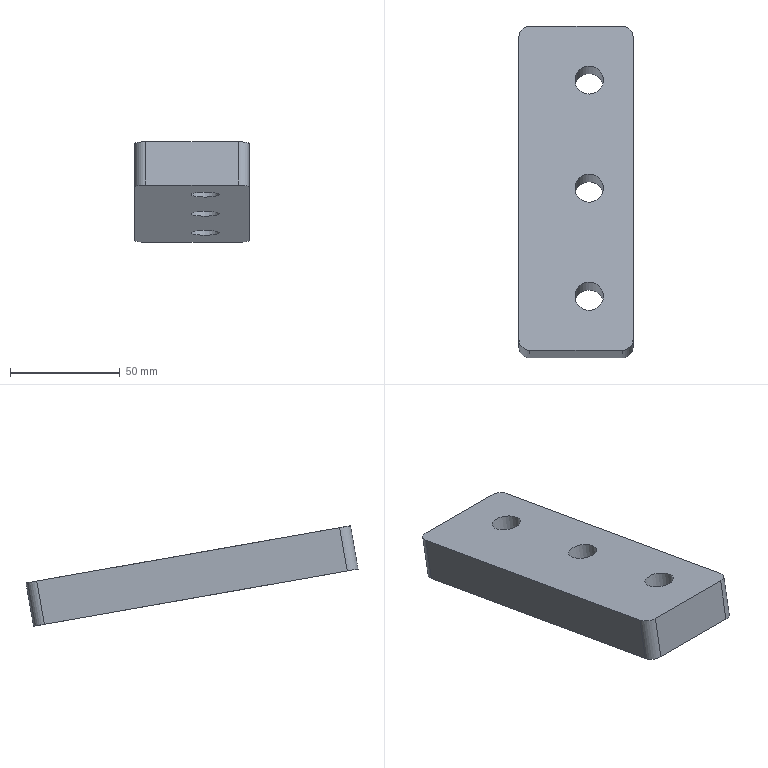Part | NX | features MAIN_BODY 2 | 1 solid | 13 faces | box 52 x 151.194 x 45.743 mm | volume 147607 mm3 | cylinder 7 | plane 6 | commonest cylinder face diameters 10 x4 13 x3
STEP:
#1=CARTESIAN_POINT('',(868.762,-740.098,-73.129));
#2=VERTEX_POINT('',#1);
#3=CARTESIAN_POINT('',(910.762,-740.098,-73.129));
#4=VERTEX_POINT('',#3);
#5=CARTESIAN_POINT('',(863.762,-740.098,-73.129));
#6=DIRECTION('',(1.,0.,0.));
#7=VECTOR('',#6,1000.);
#8=LINE('',#5,#7);
#9=EDGE_CURVE('',#2,#4,#8,.T.);
#10=ORIENTED_EDGE('',*,*,#9,.F.);
#11=CARTESIAN_POINT('',(868.762,-736.625,-53.433));
#12=VERTEX_POINT('',#11);
#13=CARTESIAN_POINT('',(868.762,-736.625,-53.433));
#14=DIRECTION('',(0.,-0.1736,-0.9848));
#15=VECTOR('',#14,1000.);
#16=LINE('',#13,#15);
#17=EDGE_CURVE('',#2,#12,#16,.F.);
#18=ORIENTED_EDGE('',*,*,#17,.T.);
#19=CARTESIAN_POINT('',(910.762,-736.625,-53.433));
#20=VERTEX_POINT('',#19);
#21=CARTESIAN_POINT('',(863.762,-736.625,-53.433));
#22=DIRECTION('',(1.,0.,0.));
#23=VECTOR('',#22,1000.);
#24=LINE('',#21,#23);
#25=EDGE_CURVE('',#12,#20,#24,.T.);
#26=ORIENTED_EDGE('',*,*,#25,.T.);
#27=CARTESIAN_POINT('',(910.762,-736.625,-53.433));
#28=DIRECTION('',(0.,-0.1736,-0.9848));
#29=VECTOR('',#28,1000.);
#30=LINE('',#27,#29);
#31=EDGE_CURVE('',#20,#4,#30,.T.);
#32=ORIENTED_EDGE('',*,*,#31,.T.);
#33=EDGE_LOOP('',(#10,#18,#26,#32));
#34=FACE_BOUND('',#33,.T.);
#35=CARTESIAN_POINT('',(863.762,-736.625,-53.433));
#36=DIRECTION('',(0.,0.9848,-0.1736));
#37=DIRECTION('',(-1.,0.,0.));
#38=AXIS2_PLACEMENT_3D('',#35,#36,#37);
#39=PLANE('',#38);
#40=ADVANCED_FACE('',(#34),#39,.T.);
#41=CARTESIAN_POINT('',(915.762,-745.022,-72.261));
#42=VERTEX_POINT('',#41);
#43=CARTESIAN_POINT('',(915.762,-882.895,-47.95));
#44=VERTEX_POINT('',#43);
#45=CARTESIAN_POINT('',(915.762,-740.098,-73.129));
#46=DIRECTION('',(0.,-0.9848,0.1736));
#47=VECTOR('',#46,1000.);
#48=LINE('',#45,#47);
#49=EDGE_CURVE('',#42,#44,#48,.T.);
#50=ORIENTED_EDGE('',*,*,#49,.F.);
#51=CARTESIAN_POINT('',(915.762,-741.549,-52.564));
#52=VERTEX_POINT('',#51);
#53=CARTESIAN_POINT('',(915.762,-741.549,-52.564));
#54=DIRECTION('',(0.,-0.1736,-0.9848));
#55=VECTOR('',#54,1000.);
#56=LINE('',#53,#55);
#57=EDGE_CURVE('',#42,#52,#56,.F.);
#58=ORIENTED_EDGE('',*,*,#57,.T.);
#59=CARTESIAN_POINT('',(915.762,-879.422,-28.254));
#60=VERTEX_POINT('',#59);
#61=CARTESIAN_POINT('',(915.762,-736.625,-53.433));
#62=DIRECTION('',(0.,-0.9848,0.1736));
#63=VECTOR('',#62,1000.);
#64=LINE('',#61,#63);
#65=EDGE_CURVE('',#52,#60,#64,.T.);
#66=ORIENTED_EDGE('',*,*,#65,.T.);
#67=CARTESIAN_POINT('',(915.762,-879.422,-28.254));
#68=DIRECTION('',(0.,-0.1736,-0.9848));
#69=VECTOR('',#68,1000.);
#70=LINE('',#67,#69);
#71=EDGE_CURVE('',#60,#44,#70,.T.);
#72=ORIENTED_EDGE('',*,*,#71,.T.);
#73=EDGE_LOOP('',(#50,#58,#66,#72));
#74=FACE_BOUND('',#73,.T.);
#75=CARTESIAN_POINT('',(915.762,-736.625,-53.433));
#76=DIRECTION('',(1.,0.,0.));
#77=DIRECTION('',(0.,0.9848,-0.1736));
#78=AXIS2_PLACEMENT_3D('',#75,#76,#77);
#79=PLANE('',#78);
#80=ADVANCED_FACE('',(#74),#79,.T.);
#81=CARTESIAN_POINT('',(863.762,-879.422,-28.254));
#82=VERTEX_POINT('',#81);
#83=CARTESIAN_POINT('',(863.762,-741.549,-52.564));
#84=VERTEX_POINT('',#83);
#85=CARTESIAN_POINT('',(863.762,-810.485,-40.409));
#86=DIRECTION('',(0.,0.9848,-0.1736));
#87=VECTOR('',#86,1000.);
#88=LINE('',#85,#87);
#89=EDGE_CURVE('',#82,#84,#88,.T.);
#90=ORIENTED_EDGE('',*,*,#89,.T.);
#91=CARTESIAN_POINT('',(863.762,-745.022,-72.261));
#92=VERTEX_POINT('',#91);
#93=CARTESIAN_POINT('',(863.762,-741.549,-52.564));
#94=DIRECTION('',(0.,-0.1736,-0.9848));
#95=VECTOR('',#94,1000.);
#96=LINE('',#93,#95);
#97=EDGE_CURVE('',#84,#92,#96,.T.);
#98=ORIENTED_EDGE('',*,*,#97,.T.);
#99=CARTESIAN_POINT('',(863.762,-882.895,-47.95));
#100=VERTEX_POINT('',#99);
#101=CARTESIAN_POINT('',(863.762,-813.958,-60.105));
#102=DIRECTION('',(0.,0.9848,-0.1736));
#103=VECTOR('',#102,1000.);
#104=LINE('',#101,#103);
#105=EDGE_CURVE('',#100,#92,#104,.T.);
#106=ORIENTED_EDGE('',*,*,#105,.F.);
#107=CARTESIAN_POINT('',(863.762,-879.422,-28.254));
#108=DIRECTION('',(0.,-0.1736,-0.9848));
#109=VECTOR('',#108,1000.);
#110=LINE('',#107,#109);
#111=EDGE_CURVE('',#100,#82,#110,.F.);
#112=ORIENTED_EDGE('',*,*,#111,.T.);
#113=EDGE_LOOP('',(#90,#98,#106,#112));
#114=FACE_BOUND('',#113,.T.);
#115=CARTESIAN_POINT('',(863.762,-810.485,-40.409));
#116=DIRECTION('',(-1.,0.,0.));
#117=DIRECTION('',(0.,-0.9848,0.1736));
#118=AXIS2_PLACEMENT_3D('',#115,#116,#117);
#119=PLANE('',#118);
#120=ADVANCED_FACE('',(#114),#119,.T.);
#121=ORIENTED_EDGE('',*,*,#25,.F.);
#122=CARTESIAN_POINT('',(868.762,-741.549,-52.564));
#123=DIRECTION('',(0.,-0.1736,-0.9848));
#124=DIRECTION('',(0.,-0.9848,0.1736));
#125=AXIS2_PLACEMENT_3D('',#122,#123,#124);
#126=CIRCLE('',#125,5.);
#127=EDGE_CURVE('',#12,#84,#126,.F.);
#128=ORIENTED_EDGE('',*,*,#127,.T.);
#129=ORIENTED_EDGE('',*,*,#89,.F.);
#130=CARTESIAN_POINT('',(868.762,-884.346,-27.385));
#131=VERTEX_POINT('',#130);
#132=CARTESIAN_POINT('',(868.762,-879.422,-28.254));
#133=DIRECTION('',(0.,-0.1736,-0.9848));
#134=DIRECTION('',(0.,-0.9848,0.1736));
#135=AXIS2_PLACEMENT_3D('',#132,#133,#134);
#136=CIRCLE('',#135,5.);
#137=EDGE_CURVE('',#82,#131,#136,.F.);
#138=ORIENTED_EDGE('',*,*,#137,.T.);
#139=CARTESIAN_POINT('',(910.762,-884.346,-27.385));
#140=VERTEX_POINT('',#139);
#141=CARTESIAN_POINT('',(863.762,-884.346,-27.385));
#142=DIRECTION('',(1.,0.,0.));
#143=VECTOR('',#142,1000.);
#144=LINE('',#141,#143);
#145=EDGE_CURVE('',#131,#140,#144,.T.);
#146=ORIENTED_EDGE('',*,*,#145,.T.);
#147=CARTESIAN_POINT('',(910.762,-879.422,-28.254));
#148=DIRECTION('',(0.,-0.1736,-0.9848));
#149=DIRECTION('',(0.,-0.9848,0.1736));
#150=AXIS2_PLACEMENT_3D('',#147,#148,#149);
#151=CIRCLE('',#150,5.);
#152=EDGE_CURVE('',#140,#60,#151,.F.);
#153=ORIENTED_EDGE('',*,*,#152,.T.);
#154=ORIENTED_EDGE('',*,*,#65,.F.);
#155=CARTESIAN_POINT('',(910.762,-741.549,-52.564));
#156=DIRECTION('',(0.,-0.1736,-0.9848));
#157=DIRECTION('',(0.,-0.9848,0.1736));
#158=AXIS2_PLACEMENT_3D('',#155,#156,#157);
#159=CIRCLE('',#158,5.);
#160=EDGE_CURVE('',#52,#20,#159,.F.);
#161=ORIENTED_EDGE('',*,*,#160,.T.);
#162=EDGE_LOOP('',(#121,#128,#129,#138,#146,#153,#154,#161));
#163=FACE_BOUND('',#162,.T.);
#164=CARTESIAN_POINT('',(895.762,-767.646,-47.963));
#165=VERTEX_POINT('',#164);
#166=CARTESIAN_POINT('',(895.762,-761.245,-49.091));
#167=DIRECTION('',(0.,-0.1736,-0.9848));
#168=DIRECTION('',(0.,-0.9848,0.1736));
#169=AXIS2_PLACEMENT_3D('',#166,#167,#168);
#170=CIRCLE('',#169,6.5);
#171=EDGE_CURVE('',#165,#165,#170,.T.);
#172=ORIENTED_EDGE('',*,*,#171,.T.);
#173=EDGE_LOOP('',(#172));
#174=FACE_BOUND('',#173,.T.);
#175=CARTESIAN_POINT('',(895.762,-816.887,-39.28));
#176=VERTEX_POINT('',#175);
#177=CARTESIAN_POINT('',(895.762,-810.485,-40.409));
#178=DIRECTION('',(0.,-0.1736,-0.9848));
#179=DIRECTION('',(0.,-0.9848,0.1736));
#180=AXIS2_PLACEMENT_3D('',#177,#178,#179);
#181=CIRCLE('',#180,6.5);
#182=EDGE_CURVE('',#176,#176,#181,.T.);
#183=ORIENTED_EDGE('',*,*,#182,.T.);
#184=EDGE_LOOP('',(#183));
#185=FACE_BOUND('',#184,.T.);
#186=CARTESIAN_POINT('',(895.762,-853.325,-32.855));
#187=VERTEX_POINT('',#186);
#188=CARTESIAN_POINT('',(895.762,-859.726,-31.727));
#189=DIRECTION('',(0.,0.1736,0.9848));
#190=DIRECTION('',(0.,0.9848,-0.1736));
#191=AXIS2_PLACEMENT_3D('',#188,#189,#190);
#192=CIRCLE('',#191,6.5);
#193=EDGE_CURVE('',#187,#187,#192,.T.);
#194=ORIENTED_EDGE('',*,*,#193,.F.);
#195=EDGE_LOOP('',(#194));
#196=FACE_BOUND('',#195,.T.);
#197=CARTESIAN_POINT('',(915.762,-736.625,-53.433));
#198=DIRECTION('',(0.,-0.1736,-0.9848));
#199=DIRECTION('',(0.,-0.9848,0.1736));
#200=AXIS2_PLACEMENT_3D('',#197,#198,#199);
#201=PLANE('',#200);
#202=ADVANCED_FACE('',(#163,#174,#185,#196),#201,.F.);
#203=ORIENTED_EDGE('',*,*,#105,.T.);
#204=CARTESIAN_POINT('',(868.762,-745.022,-72.261));
#205=DIRECTION('',(0.,-0.1736,-0.9848));
#206=DIRECTION('',(0.,-0.9848,0.1736));
#207=AXIS2_PLACEMENT_3D('',#204,#205,#206);
#208=CIRCLE('',#207,5.);
#209=EDGE_CURVE('',#92,#2,#208,.T.);
#210=ORIENTED_EDGE('',*,*,#209,.T.);
#211=ORIENTED_EDGE('',*,*,#9,.T.);
#212=CARTESIAN_POINT('',(910.762,-745.022,-72.261));
#213=DIRECTION('',(0.,-0.1736,-0.9848));
#214=DIRECTION('',(0.,-0.9848,0.1736));
#215=AXIS2_PLACEMENT_3D('',#212,#213,#214);
#216=CIRCLE('',#215,5.);
#217=EDGE_CURVE('',#4,#42,#216,.T.);
#218=ORIENTED_EDGE('',*,*,#217,.T.);
#219=ORIENTED_EDGE('',*,*,#49,.T.);
#220=CARTESIAN_POINT('',(910.762,-887.819,-47.082));
#221=VERTEX_POINT('',#220);
#222=CARTESIAN_POINT('',(910.762,-882.895,-47.95));
#223=DIRECTION('',(0.,-0.1736,-0.9848));
#224=DIRECTION('',(0.,-0.9848,0.1736));
#225=AXIS2_PLACEMENT_3D('',#222,#223,#224);
#226=CIRCLE('',#225,5.);
#227=EDGE_CURVE('',#44,#221,#226,.T.);
#228=ORIENTED_EDGE('',*,*,#227,.T.);
#229=CARTESIAN_POINT('',(868.762,-887.819,-47.082));
#230=VERTEX_POINT('',#229);
#231=CARTESIAN_POINT('',(863.762,-887.819,-47.082));
#232=DIRECTION('',(1.,0.,0.));
#233=VECTOR('',#232,1000.);
#234=LINE('',#231,#233);
#235=EDGE_CURVE('',#230,#221,#234,.T.);
#236=ORIENTED_EDGE('',*,*,#235,.F.);
#237=CARTESIAN_POINT('',(868.762,-882.895,-47.95));
#238=DIRECTION('',(0.,-0.1736,-0.9848));
#239=DIRECTION('',(0.,-0.9848,0.1736));
#240=AXIS2_PLACEMENT_3D('',#237,#238,#239);
#241=CIRCLE('',#240,5.);
#242=EDGE_CURVE('',#230,#100,#241,.T.);
#243=ORIENTED_EDGE('',*,*,#242,.T.);
#244=EDGE_LOOP('',(#203,#210,#211,#218,#219,#228,#236,#243));
#245=FACE_BOUND('',#244,.T.);
#246=CARTESIAN_POINT('',(895.762,-820.36,-58.976));
#247=VERTEX_POINT('',#246);
#248=CARTESIAN_POINT('',(895.762,-813.958,-60.105));
#249=DIRECTION('',(0.,-0.1736,-0.9848));
#250=DIRECTION('',(0.,-0.9848,0.1736));
#251=AXIS2_PLACEMENT_3D('',#248,#249,#250);
#252=CIRCLE('',#251,6.5);
#253=EDGE_CURVE('',#247,#247,#252,.T.);
#254=ORIENTED_EDGE('',*,*,#253,.F.);
#255=EDGE_LOOP('',(#254));
#256=FACE_BOUND('',#255,.T.);
#257=CARTESIAN_POINT('',(895.762,-771.119,-67.659));
#258=VERTEX_POINT('',#257);
#259=CARTESIAN_POINT('',(895.762,-764.718,-68.788));
#260=DIRECTION('',(0.,-0.1736,-0.9848));
#261=DIRECTION('',(0.,-0.9848,0.1736));
#262=AXIS2_PLACEMENT_3D('',#259,#260,#261);
#263=CIRCLE('',#262,6.5);
#264=EDGE_CURVE('',#258,#258,#263,.T.);
#265=ORIENTED_EDGE('',*,*,#264,.F.);
#266=EDGE_LOOP('',(#265));
#267=FACE_BOUND('',#266,.T.);
#268=CARTESIAN_POINT('',(895.762,-856.798,-52.551));
#269=VERTEX_POINT('',#268);
#270=CARTESIAN_POINT('',(895.762,-863.199,-51.423));
#271=DIRECTION('',(0.,0.1736,0.9848));
#272=DIRECTION('',(0.,0.9848,-0.1736));
#273=AXIS2_PLACEMENT_3D('',#270,#271,#272);
#274=CIRCLE('',#273,6.5);
#275=EDGE_CURVE('',#269,#269,#274,.T.);
#276=ORIENTED_EDGE('',*,*,#275,.T.);
#277=EDGE_LOOP('',(#276));
#278=FACE_BOUND('',#277,.T.);
#279=CARTESIAN_POINT('',(915.762,-740.098,-73.129));
#280=DIRECTION('',(0.,-0.1736,-0.9848));
#281=DIRECTION('',(0.,-0.9848,0.1736));
#282=AXIS2_PLACEMENT_3D('',#279,#280,#281);
#283=PLANE('',#282);
#284=ADVANCED_FACE('',(#245,#256,#267,#278),#283,.T.);
#285=ORIENTED_EDGE('',*,*,#264,.T.);
#286=EDGE_LOOP('',(#285));
#287=FACE_BOUND('',#286,.T.);
#288=ORIENTED_EDGE('',*,*,#171,.F.);
#289=EDGE_LOOP('',(#288));
#290=FACE_BOUND('',#289,.T.);
#291=CARTESIAN_POINT('',(895.762,-761.245,-49.091));
#292=DIRECTION('',(0.,-0.1736,-0.9848));
#293=DIRECTION('',(0.,-0.9848,0.1736));
#294=AXIS2_PLACEMENT_3D('',#291,#292,#293);
#295=CYLINDRICAL_SURFACE('',#294,6.5);
#296=ADVANCED_FACE('',(#287,#290),#295,.F.);
#297=ORIENTED_EDGE('',*,*,#253,.T.);
#298=EDGE_LOOP('',(#297));
#299=FACE_BOUND('',#298,.T.);
#300=ORIENTED_EDGE('',*,*,#182,.F.);
#301=EDGE_LOOP('',(#300));
#302=FACE_BOUND('',#301,.T.);
#303=CARTESIAN_POINT('',(895.762,-810.485,-40.409));
#304=DIRECTION('',(0.,-0.1736,-0.9848));
#305=DIRECTION('',(0.,-0.9848,0.1736));
#306=AXIS2_PLACEMENT_3D('',#303,#304,#305);
#307=CYLINDRICAL_SURFACE('',#306,6.5);
#308=ADVANCED_FACE('',(#299,#302),#307,.F.);
#309=ORIENTED_EDGE('',*,*,#145,.F.);
#310=CARTESIAN_POINT('',(868.762,-884.346,-27.385));
#311=DIRECTION('',(0.,-0.1736,-0.9848));
#312=VECTOR('',#311,1000.);
#313=LINE('',#310,#312);
#314=EDGE_CURVE('',#131,#230,#313,.T.);
#315=ORIENTED_EDGE('',*,*,#314,.T.);
#316=ORIENTED_EDGE('',*,*,#235,.T.);
#317=CARTESIAN_POINT('',(910.762,-884.346,-27.385));
#318=DIRECTION('',(0.,-0.1736,-0.9848));
#319=VECTOR('',#318,1000.);
#320=LINE('',#317,#319);
#321=EDGE_CURVE('',#221,#140,#320,.F.);
#322=ORIENTED_EDGE('',*,*,#321,.T.);
#323=EDGE_LOOP('',(#309,#315,#316,#322));
#324=FACE_BOUND('',#323,.T.);
#325=CARTESIAN_POINT('',(863.762,-884.346,-27.385));
#326=DIRECTION('',(0.,-0.9848,0.1736));
#327=DIRECTION('',(-1.,0.,0.));
#328=AXIS2_PLACEMENT_3D('',#325,#326,#327);
#329=PLANE('',#328);
#330=ADVANCED_FACE('',(#324),#329,.T.);
#331=ORIENTED_EDGE('',*,*,#275,.F.);
#332=EDGE_LOOP('',(#331));
#333=FACE_BOUND('',#332,.T.);
#334=ORIENTED_EDGE('',*,*,#193,.T.);
#335=EDGE_LOOP('',(#334));
#336=FACE_BOUND('',#335,.T.);
#337=CARTESIAN_POINT('',(895.762,-859.726,-31.727));
#338=DIRECTION('',(0.,-0.1736,-0.9848));
#339=DIRECTION('',(0.,0.9848,-0.1736));
#340=AXIS2_PLACEMENT_3D('',#337,#338,#339);
#341=CYLINDRICAL_SURFACE('',#340,6.5);
#342=ADVANCED_FACE('',(#333,#336),#341,.F.);
#343=ORIENTED_EDGE('',*,*,#127,.F.);
#344=ORIENTED_EDGE('',*,*,#17,.F.);
#345=ORIENTED_EDGE('',*,*,#209,.F.);
#346=ORIENTED_EDGE('',*,*,#97,.F.);
#347=EDGE_LOOP('',(#343,#344,#345,#346));
#348=FACE_BOUND('',#347,.T.);
#349=CARTESIAN_POINT('',(868.762,-741.549,-52.564));
#350=DIRECTION('',(0.,-0.1736,-0.9848));
#351=DIRECTION('',(0.,-0.9848,0.1736));
#352=AXIS2_PLACEMENT_3D('',#349,#350,#351);
#353=CYLINDRICAL_SURFACE('',#352,5.);
#354=ADVANCED_FACE('',(#348),#353,.T.);
#355=ORIENTED_EDGE('',*,*,#160,.F.);
#356=ORIENTED_EDGE('',*,*,#57,.F.);
#357=ORIENTED_EDGE('',*,*,#217,.F.);
#358=ORIENTED_EDGE('',*,*,#31,.F.);
#359=EDGE_LOOP('',(#355,#356,#357,#358));
#360=FACE_BOUND('',#359,.T.);
#361=CARTESIAN_POINT('',(910.762,-741.549,-52.564));
#362=DIRECTION('',(0.,-0.1736,-0.9848));
#363=DIRECTION('',(0.,-0.9848,0.1736));
#364=AXIS2_PLACEMENT_3D('',#361,#362,#363);
#365=CYLINDRICAL_SURFACE('',#364,5.);
#366=ADVANCED_FACE('',(#360),#365,.T.);
#367=ORIENTED_EDGE('',*,*,#137,.F.);
#368=ORIENTED_EDGE('',*,*,#111,.F.);
#369=ORIENTED_EDGE('',*,*,#242,.F.);
#370=ORIENTED_EDGE('',*,*,#314,.F.);
#371=EDGE_LOOP('',(#367,#368,#369,#370));
#372=FACE_BOUND('',#371,.T.);
#373=CARTESIAN_POINT('',(868.762,-879.422,-28.254));
#374=DIRECTION('',(0.,-0.1736,-0.9848));
#375=DIRECTION('',(0.,-0.9848,0.1736));
#376=AXIS2_PLACEMENT_3D('',#373,#374,#375);
#377=CYLINDRICAL_SURFACE('',#376,5.);
#378=ADVANCED_FACE('',(#372),#377,.T.);
#379=ORIENTED_EDGE('',*,*,#152,.F.);
#380=ORIENTED_EDGE('',*,*,#321,.F.);
#381=ORIENTED_EDGE('',*,*,#227,.F.);
#382=ORIENTED_EDGE('',*,*,#71,.F.);
#383=EDGE_LOOP('',(#379,#380,#381,#382));
#384=FACE_BOUND('',#383,.T.);
#385=CARTESIAN_POINT('',(910.762,-879.422,-28.254));
#386=DIRECTION('',(0.,-0.1736,-0.9848));
#387=DIRECTION('',(0.,-0.9848,0.1736));
#388=AXIS2_PLACEMENT_3D('',#385,#386,#387);
#389=CYLINDRICAL_SURFACE('',#388,5.);
#390=ADVANCED_FACE('',(#384),#389,.T.);
#391=CLOSED_SHELL('',(#40,#80,#120,#202,#284,#296,#308,#330,#342,#354,#366,#378,#390));
#392=MANIFOLD_SOLID_BREP('',#391);
#393=(LENGTH_UNIT()NAMED_UNIT(*)SI_UNIT(.MILLI.,.METRE.));
#394=UNCERTAINTY_MEASURE_WITH_UNIT(LENGTH_MEASURE(0.00001),#393,'','');
#395=(NAMED_UNIT(*)PLANE_ANGLE_UNIT()SI_UNIT($,.RADIAN.));
#396=(NAMED_UNIT(*)SI_UNIT($,.STERADIAN.)SOLID_ANGLE_UNIT());
#397=(GEOMETRIC_REPRESENTATION_CONTEXT(3)GLOBAL_UNCERTAINTY_ASSIGNED_CONTEXT((#394))GLOBAL_UNIT_ASSIGNED_CONTEXT((#393,#395,#396))REPRESENTATION_CONTEXT('',''));
#398=ADVANCED_BREP_SHAPE_REPRESENTATION('',(#392),#397);